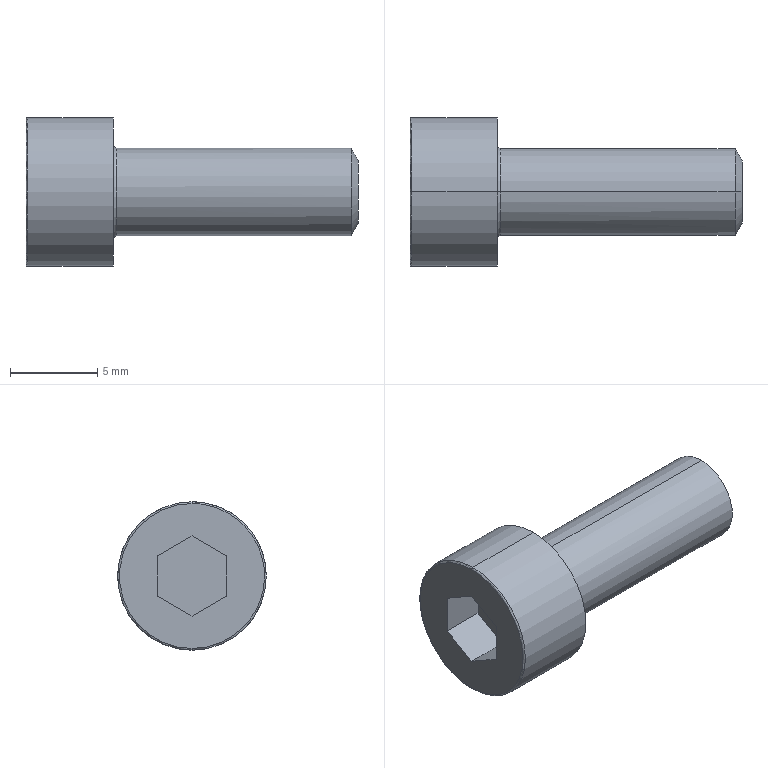Part | STEP file | 103000006185 | 1 solid | 20 faces | box 19 x 8.5 x 8.5 mm | volume 522.658 mm3 | plane 10 | torus 4 | cylinder 4 | cone 2 | commonest cylinder face diameters 5 x2 8.5 x2
STEP:
#1=CARTESIAN_POINT('',(0.,0.,4.15));
#2=VERTEX_POINT('',#1);
#3=CARTESIAN_POINT('',(0.,0.,-4.15));
#4=VERTEX_POINT('',#3);
#5=CARTESIAN_POINT('',(0.,0.,0.));
#6=DIRECTION('',(1.,0.,0.));
#7=AXIS2_PLACEMENT_3D('',#5,#6,$);
#8=CIRCLE('',#7,4.15);
#9=EDGE_CURVE('',#2,#4,#8,.F.);
#10=ORIENTED_EDGE('',*,*,#9,.F.);
#11=CARTESIAN_POINT('',(0.1,0.,4.25));
#12=VERTEX_POINT('',#11);
#13=CARTESIAN_POINT('',(0.1,0.,4.15));
#14=DIRECTION('',(0.,1.,0.));
#15=AXIS2_PLACEMENT_3D('',#13,#14,$);
#16=CIRCLE('',#15,0.1);
#17=EDGE_CURVE('',#2,#12,#16,.T.);
#18=ORIENTED_EDGE('',*,*,#17,.T.);
#19=CARTESIAN_POINT('',(0.1,0.,-4.25));
#20=VERTEX_POINT('',#19);
#21=CARTESIAN_POINT('',(0.1,0.,0.));
#22=DIRECTION('',(1.,0.,0.));
#23=AXIS2_PLACEMENT_3D('',#21,#22,$);
#24=CIRCLE('',#23,4.25);
#25=EDGE_CURVE('',#20,#12,#24,.T.);
#26=ORIENTED_EDGE('',*,*,#25,.F.);
#27=CARTESIAN_POINT('',(0.1,0.,-4.15));
#28=DIRECTION('',(0.,-1.,0.));
#29=AXIS2_PLACEMENT_3D('',#27,#28,$);
#30=CIRCLE('',#29,0.1);
#31=EDGE_CURVE('',#4,#20,#30,.T.);
#32=ORIENTED_EDGE('',*,*,#31,.F.);
#33=EDGE_LOOP('',(#10,#18,#26,#32));
#34=FACE_OUTER_BOUND('',#33,.T.);
#35=CARTESIAN_POINT('',(0.1,0.,0.));
#36=DIRECTION('',(1.,0.,0.));
#37=DIRECTION('',(0.,0.,-1.));
#38=AXIS2_PLACEMENT_3D('',#35,#36,#37);
#39=TOROIDAL_SURFACE('',#38,4.15,0.1);
#40=ADVANCED_FACE('',(#34),#39,.T.);
#41=CARTESIAN_POINT('',(0.,0.,-4.15));
#42=CARTESIAN_POINT('',(0.,-0.3992,-4.15));
#43=CARTESIAN_POINT('',(0.,-0.7984,-4.102));
#44=CARTESIAN_POINT('',(0.,-1.19,-4.006));
#45=CARTESIAN_POINT('',(0.,-1.942,-3.722));
#46=CARTESIAN_POINT('',(0.,-2.606,-3.267));
#47=CARTESIAN_POINT('',(0.,-2.908,-3.001));
#48=CARTESIAN_POINT('',(0.,-3.444,-2.401));
#49=CARTESIAN_POINT('',(0.,-3.821,-1.691));
#50=CARTESIAN_POINT('',(0.,-3.967,-1.315));
#51=CARTESIAN_POINT('',(0.,-4.164,-0.5355));
#52=CARTESIAN_POINT('',(0.,-4.17,0.2686));
#53=CARTESIAN_POINT('',(0.,-4.125,0.6692));
#54=CARTESIAN_POINT('',(0.,-3.939,1.452));
#55=CARTESIAN_POINT('',(0.,-3.573,2.167));
#56=CARTESIAN_POINT('',(0.,-3.347,2.502));
#57=CARTESIAN_POINT('',(0.,-2.821,3.109));
#58=CARTESIAN_POINT('',(0.,-2.165,3.575));
#59=CARTESIAN_POINT('',(0.,-1.81,3.766));
#60=CARTESIAN_POINT('',(0.,-1.237,3.992));
#61=CARTESIAN_POINT('',(0.,-0.6358,4.109));
#62=CARTESIAN_POINT('',(0.,-0.4247,4.136));
#63=CARTESIAN_POINT('',(0.,-0.2123,4.15));
#64=CARTESIAN_POINT('',(0.,0.,4.15));
#65=B_SPLINE_CURVE_WITH_KNOTS('',5,(#41,#42,#43,#44,#45,#46,#47,#48,#49,#50,#51,#52,#53,#54,#55,#56,#57,#58,#59,#60,#61,#62,#63,#64),.UNSPECIFIED.,.F.,.U.,(6,3,3,3,3,3,3,6),(0.,2.823,5.645,8.468,11.291,14.114,16.936,18.438),.UNSPECIFIED.);
#66=EDGE_CURVE('',#4,#2,#65,.T.);
#67=ORIENTED_EDGE('',*,*,#66,.T.);
#68=ORIENTED_EDGE('',*,*,#9,.T.);
#69=EDGE_LOOP('',(#67,#68));
#70=FACE_OUTER_BOUND('',#69,.T.);
#71=CARTESIAN_POINT('',(0.,0.,2.29));
#72=VERTEX_POINT('',#71);
#73=CARTESIAN_POINT('',(0.,1.983,1.145));
#74=VERTEX_POINT('',#73);
#75=CARTESIAN_POINT('',(0.,0.9916,1.717));
#76=DIRECTION('',(0.,0.866,-0.5));
#77=VECTOR('',#76,1.);
#78=LINE('',#75,#77);
#79=EDGE_CURVE('',#72,#74,#78,.T.);
#80=ORIENTED_EDGE('',*,*,#79,.F.);
#81=CARTESIAN_POINT('',(0.,-1.983,1.145));
#82=VERTEX_POINT('',#81);
#83=CARTESIAN_POINT('',(0.,-0.9916,1.717));
#84=DIRECTION('',(0.,0.866,0.5));
#85=VECTOR('',#84,1.);
#86=LINE('',#83,#85);
#87=EDGE_CURVE('',#82,#72,#86,.T.);
#88=ORIENTED_EDGE('',*,*,#87,.F.);
#89=CARTESIAN_POINT('',(0.,-1.983,-1.145));
#90=VERTEX_POINT('',#89);
#91=CARTESIAN_POINT('',(0.,-1.983,0.));
#92=DIRECTION('',(0.,0.,1.));
#93=VECTOR('',#92,1.);
#94=LINE('',#91,#93);
#95=EDGE_CURVE('',#90,#82,#94,.T.);
#96=ORIENTED_EDGE('',*,*,#95,.F.);
#97=CARTESIAN_POINT('',(0.,0.,-2.29));
#98=VERTEX_POINT('',#97);
#99=CARTESIAN_POINT('',(0.,-0.9916,-1.717));
#100=DIRECTION('',(0.,-0.866,0.5));
#101=VECTOR('',#100,1.);
#102=LINE('',#99,#101);
#103=EDGE_CURVE('',#98,#90,#102,.T.);
#104=ORIENTED_EDGE('',*,*,#103,.F.);
#105=CARTESIAN_POINT('',(0.,1.983,-1.145));
#106=VERTEX_POINT('',#105);
#107=CARTESIAN_POINT('',(0.,0.9916,-1.717));
#108=DIRECTION('',(0.,-0.866,-0.5));
#109=VECTOR('',#108,1.);
#110=LINE('',#107,#109);
#111=EDGE_CURVE('',#106,#98,#110,.T.);
#112=ORIENTED_EDGE('',*,*,#111,.F.);
#113=CARTESIAN_POINT('',(0.,1.983,0.));
#114=DIRECTION('',(0.,0.,-1.));
#115=VECTOR('',#114,1.);
#116=LINE('',#113,#115);
#117=EDGE_CURVE('',#74,#106,#116,.T.);
#118=ORIENTED_EDGE('',*,*,#117,.F.);
#119=EDGE_LOOP('',(#80,#88,#96,#104,#112,#118));
#120=FACE_BOUND('',#119,.T.);
#121=CARTESIAN_POINT('',(0.,0.,0.));
#122=DIRECTION('',(1.,0.,0.));
#123=DIRECTION('',(0.,0.,-1.));
#124=AXIS2_PLACEMENT_3D('',#121,#122,#123);
#125=PLANE('',#124);
#126=ADVANCED_FACE('',(#70,#120),#125,.F.);
#127=ORIENTED_EDGE('',*,*,#17,.F.);
#128=ORIENTED_EDGE('',*,*,#66,.F.);
#129=ORIENTED_EDGE('',*,*,#31,.T.);
#130=CARTESIAN_POINT('',(0.1,0.,0.));
#131=DIRECTION('',(1.,0.,0.));
#132=AXIS2_PLACEMENT_3D('',#130,#131,$);
#133=CIRCLE('',#132,4.25);
#134=EDGE_CURVE('',#12,#20,#133,.T.);
#135=ORIENTED_EDGE('',*,*,#134,.F.);
#136=EDGE_LOOP('',(#127,#128,#129,#135));
#137=FACE_OUTER_BOUND('',#136,.T.);
#138=CARTESIAN_POINT('',(0.1,0.,0.));
#139=DIRECTION('',(1.,0.,0.));
#140=DIRECTION('',(0.,0.,1.));
#141=AXIS2_PLACEMENT_3D('',#138,#139,#140);
#142=TOROIDAL_SURFACE('',#141,4.15,0.1);
#143=ADVANCED_FACE('',(#137),#142,.T.);
#144=CARTESIAN_POINT('',(5.,0.,4.25));
#145=VERTEX_POINT('',#144);
#146=CARTESIAN_POINT('',(5.,0.,-4.25));
#147=VERTEX_POINT('',#146);
#148=CARTESIAN_POINT('',(5.,0.,0.));
#149=DIRECTION('',(-1.,0.,0.));
#150=AXIS2_PLACEMENT_3D('',#148,#149,$);
#151=CIRCLE('',#150,4.25);
#152=EDGE_CURVE('',#145,#147,#151,.T.);
#153=ORIENTED_EDGE('',*,*,#152,.T.);
#154=CARTESIAN_POINT('',(0.,0.,-4.25));
#155=DIRECTION('',(-1.,0.,0.));
#156=VECTOR('',#155,1.);
#157=LINE('',#154,#156);
#158=EDGE_CURVE('',#147,#20,#157,.T.);
#159=ORIENTED_EDGE('',*,*,#158,.T.);
#160=ORIENTED_EDGE('',*,*,#25,.T.);
#161=CARTESIAN_POINT('',(0.,0.,4.25));
#162=DIRECTION('',(-1.,0.,0.));
#163=VECTOR('',#162,1.);
#164=LINE('',#161,#163);
#165=EDGE_CURVE('',#145,#12,#164,.T.);
#166=ORIENTED_EDGE('',*,*,#165,.F.);
#167=EDGE_LOOP('',(#153,#159,#160,#166));
#168=FACE_OUTER_BOUND('',#167,.T.);
#169=CARTESIAN_POINT('',(0.,0.,0.));
#170=DIRECTION('',(-1.,0.,0.));
#171=DIRECTION('',(0.,0.,1.));
#172=AXIS2_PLACEMENT_3D('',#169,#170,#171);
#173=CYLINDRICAL_SURFACE('',#172,4.25);
#174=ADVANCED_FACE('',(#168),#173,.T.);
#175=ORIENTED_EDGE('',*,*,#79,.T.);
#176=CARTESIAN_POINT('',(2.5,1.983,1.145));
#177=VERTEX_POINT('',#176);
#178=CARTESIAN_POINT('',(1.25,1.983,1.145));
#179=DIRECTION('',(-1.,0.,0.));
#180=VECTOR('',#179,1.);
#181=LINE('',#178,#180);
#182=EDGE_CURVE('',#177,#74,#181,.T.);
#183=ORIENTED_EDGE('',*,*,#182,.F.);
#184=CARTESIAN_POINT('',(2.5,-0.000000001,2.29));
#185=VERTEX_POINT('',#184);
#186=CARTESIAN_POINT('',(2.5,0.9916,1.718));
#187=DIRECTION('',(0.,0.866,-0.5));
#188=VECTOR('',#187,1.);
#189=LINE('',#186,#188);
#190=EDGE_CURVE('',#185,#177,#189,.T.);
#191=ORIENTED_EDGE('',*,*,#190,.F.);
#192=CARTESIAN_POINT('',(1.25,0.,2.29));
#193=DIRECTION('',(-1.,0.,0.));
#194=VECTOR('',#193,1.);
#195=LINE('',#192,#194);
#196=EDGE_CURVE('',#185,#72,#195,.T.);
#197=ORIENTED_EDGE('',*,*,#196,.T.);
#198=EDGE_LOOP('',(#175,#183,#191,#197));
#199=FACE_OUTER_BOUND('',#198,.T.);
#200=CARTESIAN_POINT('',(2.5,0.,2.29));
#201=DIRECTION('',(0.,0.5,0.866));
#202=DIRECTION('',(0.,-0.866,0.5));
#203=AXIS2_PLACEMENT_3D('',#200,#201,#202);
#204=PLANE('',#203);
#205=ADVANCED_FACE('',(#199),#204,.F.);
#206=ORIENTED_EDGE('',*,*,#87,.T.);
#207=ORIENTED_EDGE('',*,*,#196,.F.);
#208=CARTESIAN_POINT('',(2.5,-1.983,1.145));
#209=VERTEX_POINT('',#208);
#210=CARTESIAN_POINT('',(2.5,-0.9916,1.717));
#211=DIRECTION('',(0.,0.866,0.5));
#212=VECTOR('',#211,1.);
#213=LINE('',#210,#212);
#214=EDGE_CURVE('',#209,#185,#213,.T.);
#215=ORIENTED_EDGE('',*,*,#214,.F.);
#216=CARTESIAN_POINT('',(1.25,-1.983,1.145));
#217=DIRECTION('',(-1.,0.,0.));
#218=VECTOR('',#217,1.);
#219=LINE('',#216,#218);
#220=EDGE_CURVE('',#209,#82,#219,.T.);
#221=ORIENTED_EDGE('',*,*,#220,.T.);
#222=EDGE_LOOP('',(#206,#207,#215,#221));
#223=FACE_OUTER_BOUND('',#222,.T.);
#224=CARTESIAN_POINT('',(2.5,-1.983,1.145));
#225=DIRECTION('',(0.,-0.5,0.866));
#226=DIRECTION('',(0.,-0.866,-0.5));
#227=AXIS2_PLACEMENT_3D('',#224,#225,#226);
#228=PLANE('',#227);
#229=ADVANCED_FACE('',(#223),#228,.F.);
#230=ORIENTED_EDGE('',*,*,#95,.T.);
#231=ORIENTED_EDGE('',*,*,#220,.F.);
#232=CARTESIAN_POINT('',(2.5,-1.983,-1.145));
#233=VERTEX_POINT('',#232);
#234=CARTESIAN_POINT('',(2.5,-1.983,0.));
#235=DIRECTION('',(0.,0.,1.));
#236=VECTOR('',#235,1.);
#237=LINE('',#234,#236);
#238=EDGE_CURVE('',#233,#209,#237,.T.);
#239=ORIENTED_EDGE('',*,*,#238,.F.);
#240=CARTESIAN_POINT('',(1.25,-1.983,-1.145));
#241=DIRECTION('',(-1.,0.,0.));
#242=VECTOR('',#241,1.);
#243=LINE('',#240,#242);
#244=EDGE_CURVE('',#233,#90,#243,.T.);
#245=ORIENTED_EDGE('',*,*,#244,.T.);
#246=EDGE_LOOP('',(#230,#231,#239,#245));
#247=FACE_OUTER_BOUND('',#246,.T.);
#248=CARTESIAN_POINT('',(2.5,-1.983,-1.145));
#249=DIRECTION('',(0.,-1.,0.));
#250=DIRECTION('',(0.,0.,-1.));
#251=AXIS2_PLACEMENT_3D('',#248,#249,#250);
#252=PLANE('',#251);
#253=ADVANCED_FACE('',(#247),#252,.F.);
#254=ORIENTED_EDGE('',*,*,#103,.T.);
#255=ORIENTED_EDGE('',*,*,#244,.F.);
#256=CARTESIAN_POINT('',(2.5,0.,-2.29));
#257=VERTEX_POINT('',#256);
#258=CARTESIAN_POINT('',(2.5,-0.9916,-1.718));
#259=DIRECTION('',(0.,-0.866,0.5));
#260=VECTOR('',#259,1.);
#261=LINE('',#258,#260);
#262=EDGE_CURVE('',#257,#233,#261,.T.);
#263=ORIENTED_EDGE('',*,*,#262,.F.);
#264=CARTESIAN_POINT('',(1.25,0.,-2.29));
#265=DIRECTION('',(-1.,0.,0.));
#266=VECTOR('',#265,1.);
#267=LINE('',#264,#266);
#268=EDGE_CURVE('',#257,#98,#267,.T.);
#269=ORIENTED_EDGE('',*,*,#268,.T.);
#270=EDGE_LOOP('',(#254,#255,#263,#269));
#271=FACE_OUTER_BOUND('',#270,.T.);
#272=CARTESIAN_POINT('',(2.5,0.,-2.29));
#273=DIRECTION('',(0.,-0.5,-0.866));
#274=DIRECTION('',(0.,0.866,-0.5));
#275=AXIS2_PLACEMENT_3D('',#272,#273,#274);
#276=PLANE('',#275);
#277=ADVANCED_FACE('',(#271),#276,.F.);
#278=ORIENTED_EDGE('',*,*,#111,.T.);
#279=ORIENTED_EDGE('',*,*,#268,.F.);
#280=CARTESIAN_POINT('',(2.5,1.983,-1.145));
#281=VERTEX_POINT('',#280);
#282=CARTESIAN_POINT('',(2.5,0.9916,-1.717));
#283=DIRECTION('',(0.,-0.866,-0.5));
#284=VECTOR('',#283,1.);
#285=LINE('',#282,#284);
#286=EDGE_CURVE('',#281,#257,#285,.T.);
#287=ORIENTED_EDGE('',*,*,#286,.F.);
#288=CARTESIAN_POINT('',(1.25,1.983,-1.145));
#289=DIRECTION('',(-1.,0.,0.));
#290=VECTOR('',#289,1.);
#291=LINE('',#288,#290);
#292=EDGE_CURVE('',#281,#106,#291,.T.);
#293=ORIENTED_EDGE('',*,*,#292,.T.);
#294=EDGE_LOOP('',(#278,#279,#287,#293));
#295=FACE_OUTER_BOUND('',#294,.T.);
#296=CARTESIAN_POINT('',(2.5,1.983,-1.145));
#297=DIRECTION('',(0.,0.5,-0.866));
#298=DIRECTION('',(0.,0.866,0.5));
#299=AXIS2_PLACEMENT_3D('',#296,#297,#298);
#300=PLANE('',#299);
#301=ADVANCED_FACE('',(#295),#300,.F.);
#302=ORIENTED_EDGE('',*,*,#117,.T.);
#303=ORIENTED_EDGE('',*,*,#292,.F.);
#304=CARTESIAN_POINT('',(2.5,1.983,0.));
#305=DIRECTION('',(0.,0.,-1.));
#306=VECTOR('',#305,1.);
#307=LINE('',#304,#306);
#308=EDGE_CURVE('',#177,#281,#307,.T.);
#309=ORIENTED_EDGE('',*,*,#308,.F.);
#310=ORIENTED_EDGE('',*,*,#182,.T.);
#311=EDGE_LOOP('',(#302,#303,#309,#310));
#312=FACE_OUTER_BOUND('',#311,.T.);
#313=CARTESIAN_POINT('',(2.5,1.983,1.145));
#314=DIRECTION('',(0.,1.,0.));
#315=DIRECTION('',(0.,0.,1.));
#316=AXIS2_PLACEMENT_3D('',#313,#314,#315);
#317=PLANE('',#316);
#318=ADVANCED_FACE('',(#312),#317,.F.);
#319=ORIENTED_EDGE('',*,*,#158,.F.);
#320=CARTESIAN_POINT('',(5.,0.,0.));
#321=DIRECTION('',(-1.,0.,0.));
#322=AXIS2_PLACEMENT_3D('',#320,#321,$);
#323=CIRCLE('',#322,4.25);
#324=EDGE_CURVE('',#147,#145,#323,.T.);
#325=ORIENTED_EDGE('',*,*,#324,.T.);
#326=ORIENTED_EDGE('',*,*,#165,.T.);
#327=ORIENTED_EDGE('',*,*,#134,.T.);
#328=EDGE_LOOP('',(#319,#325,#326,#327));
#329=FACE_OUTER_BOUND('',#328,.T.);
#330=CARTESIAN_POINT('',(0.,0.,0.));
#331=DIRECTION('',(-1.,0.,0.));
#332=DIRECTION('',(0.,0.,-1.));
#333=AXIS2_PLACEMENT_3D('',#330,#331,#332);
#334=CYLINDRICAL_SURFACE('',#333,4.25);
#335=ADVANCED_FACE('',(#329),#334,.T.);
#336=ORIENTED_EDGE('',*,*,#152,.F.);
#337=ORIENTED_EDGE('',*,*,#324,.F.);
#338=EDGE_LOOP('',(#336,#337));
#339=FACE_OUTER_BOUND('',#338,.T.);
#340=CARTESIAN_POINT('',(5.,0.,2.7));
#341=VERTEX_POINT('',#340);
#342=CARTESIAN_POINT('',(5.,0.,-2.7));
#343=VERTEX_POINT('',#342);
#344=CARTESIAN_POINT('',(5.,0.,0.));
#345=DIRECTION('',(-1.,0.,0.));
#346=AXIS2_PLACEMENT_3D('',#344,#345,$);
#347=CIRCLE('',#346,2.7);
#348=EDGE_CURVE('',#341,#343,#347,.T.);
#349=ORIENTED_EDGE('',*,*,#348,.T.);
#350=CARTESIAN_POINT('',(5.,0.,0.));
#351=DIRECTION('',(-1.,0.,0.));
#352=AXIS2_PLACEMENT_3D('',#350,#351,$);
#353=CIRCLE('',#352,2.7);
#354=EDGE_CURVE('',#343,#341,#353,.T.);
#355=ORIENTED_EDGE('',*,*,#354,.T.);
#356=EDGE_LOOP('',(#349,#355));
#357=FACE_BOUND('',#356,.T.);
#358=CARTESIAN_POINT('',(5.,4.25,0.));
#359=DIRECTION('',(-1.,0.,0.));
#360=DIRECTION('',(0.,0.,1.));
#361=AXIS2_PLACEMENT_3D('',#358,#359,#360);
#362=PLANE('',#361);
#363=ADVANCED_FACE('',(#339,#357),#362,.F.);
#364=ORIENTED_EDGE('',*,*,#214,.T.);
#365=ORIENTED_EDGE('',*,*,#190,.T.);
#366=ORIENTED_EDGE('',*,*,#308,.T.);
#367=ORIENTED_EDGE('',*,*,#286,.T.);
#368=ORIENTED_EDGE('',*,*,#262,.T.);
#369=ORIENTED_EDGE('',*,*,#238,.T.);
#370=EDGE_LOOP('',(#364,#365,#366,#367,#368,#369));
#371=FACE_OUTER_BOUND('',#370,.T.);
#372=CARTESIAN_POINT('',(2.5,-1.983,1.145));
#373=DIRECTION('',(1.,0.,0.));
#374=DIRECTION('',(0.,0.,-1.));
#375=AXIS2_PLACEMENT_3D('',#372,#373,#374);
#376=PLANE('',#375);
#377=ADVANCED_FACE('',(#371),#376,.F.);
#378=CARTESIAN_POINT('',(5.2,0.,-2.5));
#379=VERTEX_POINT('',#378);
#380=CARTESIAN_POINT('',(5.2,0.,-2.7));
#381=DIRECTION('',(0.,1.,0.));
#382=AXIS2_PLACEMENT_3D('',#380,#381,$);
#383=CIRCLE('',#382,0.2);
#384=EDGE_CURVE('',#343,#379,#383,.T.);
#385=ORIENTED_EDGE('',*,*,#384,.F.);
#386=ORIENTED_EDGE('',*,*,#348,.F.);
#387=CARTESIAN_POINT('',(5.2,0.,2.5));
#388=VERTEX_POINT('',#387);
#389=CARTESIAN_POINT('',(5.2,0.,2.7));
#390=DIRECTION('',(0.,-1.,0.));
#391=AXIS2_PLACEMENT_3D('',#389,#390,$);
#392=CIRCLE('',#391,0.2);
#393=EDGE_CURVE('',#341,#388,#392,.T.);
#394=ORIENTED_EDGE('',*,*,#393,.T.);
#395=CARTESIAN_POINT('',(5.2,0.,0.));
#396=DIRECTION('',(-1.,0.,0.));
#397=AXIS2_PLACEMENT_3D('',#395,#396,$);
#398=CIRCLE('',#397,2.5);
#399=EDGE_CURVE('',#388,#379,#398,.T.);
#400=ORIENTED_EDGE('',*,*,#399,.T.);
#401=EDGE_LOOP('',(#385,#386,#394,#400));
#402=FACE_OUTER_BOUND('',#401,.T.);
#403=CARTESIAN_POINT('',(5.2,0.,0.));
#404=DIRECTION('',(-1.,0.,0.));
#405=DIRECTION('',(0.,0.,1.));
#406=AXIS2_PLACEMENT_3D('',#403,#404,#405);
#407=TOROIDAL_SURFACE('',#406,2.7,0.2);
#408=ADVANCED_FACE('',(#402),#407,.F.);
#409=ORIENTED_EDGE('',*,*,#354,.F.);
#410=ORIENTED_EDGE('',*,*,#384,.T.);
#411=CARTESIAN_POINT('',(5.2,0.,0.));
#412=DIRECTION('',(-1.,0.,0.));
#413=AXIS2_PLACEMENT_3D('',#411,#412,$);
#414=CIRCLE('',#413,2.5);
#415=EDGE_CURVE('',#379,#388,#414,.T.);
#416=ORIENTED_EDGE('',*,*,#415,.T.);
#417=ORIENTED_EDGE('',*,*,#393,.F.);
#418=EDGE_LOOP('',(#409,#410,#416,#417));
#419=FACE_OUTER_BOUND('',#418,.T.);
#420=CARTESIAN_POINT('',(5.2,0.,0.));
#421=DIRECTION('',(-1.,0.,0.));
#422=DIRECTION('',(0.,0.,-1.));
#423=AXIS2_PLACEMENT_3D('',#420,#421,#422);
#424=TOROIDAL_SURFACE('',#423,2.7,0.2);
#425=ADVANCED_FACE('',(#419),#424,.F.);
#426=CARTESIAN_POINT('',(18.6,0.,2.5));
#427=VERTEX_POINT('',#426);
#428=CARTESIAN_POINT('',(18.6,0.,-2.5));
#429=VERTEX_POINT('',#428);
#430=CARTESIAN_POINT('',(18.6,0.,0.));
#431=DIRECTION('',(-1.,0.,0.));
#432=AXIS2_PLACEMENT_3D('',#430,#431,$);
#433=CIRCLE('',#432,2.5);
#434=EDGE_CURVE('',#427,#429,#433,.T.);
#435=ORIENTED_EDGE('',*,*,#434,.T.);
#436=CARTESIAN_POINT('',(0.,0.,-2.5));
#437=DIRECTION('',(-1.,0.,0.));
#438=VECTOR('',#437,1.);
#439=LINE('',#436,#438);
#440=EDGE_CURVE('',#429,#379,#439,.T.);
#441=ORIENTED_EDGE('',*,*,#440,.T.);
#442=ORIENTED_EDGE('',*,*,#399,.F.);
#443=CARTESIAN_POINT('',(0.,0.,2.5));
#444=DIRECTION('',(-1.,0.,0.));
#445=VECTOR('',#444,1.);
#446=LINE('',#443,#445);
#447=EDGE_CURVE('',#427,#388,#446,.T.);
#448=ORIENTED_EDGE('',*,*,#447,.F.);
#449=EDGE_LOOP('',(#435,#441,#442,#448));
#450=FACE_OUTER_BOUND('',#449,.T.);
#451=CARTESIAN_POINT('',(0.,0.,0.));
#452=DIRECTION('',(-1.,0.,0.));
#453=DIRECTION('',(0.,0.,1.));
#454=AXIS2_PLACEMENT_3D('',#451,#452,#453);
#455=CYLINDRICAL_SURFACE('',#454,2.5);
#456=ADVANCED_FACE('',(#450),#455,.T.);
#457=ORIENTED_EDGE('',*,*,#440,.F.);
#458=CARTESIAN_POINT('',(18.6,0.,-2.5));
#459=CARTESIAN_POINT('',(18.6,-0.7854,-2.5));
#460=CARTESIAN_POINT('',(18.6,-1.571,-2.192));
#461=CARTESIAN_POINT('',(18.6,-2.192,-1.571));
#462=CARTESIAN_POINT('',(18.6,-2.808,0.));
#463=CARTESIAN_POINT('',(18.6,-2.192,1.571));
#464=CARTESIAN_POINT('',(18.6,-1.571,2.192));
#465=CARTESIAN_POINT('',(18.6,-0.7854,2.5));
#466=CARTESIAN_POINT('',(18.6,0.,2.5));
#467=B_SPLINE_CURVE_WITH_KNOTS('',5,(#458,#459,#460,#461,#462,#463,#464,#465,#466),.UNSPECIFIED.,.F.,.U.,(6,3,6),(-3.927,0.,3.927),.UNSPECIFIED.);
#468=EDGE_CURVE('',#429,#427,#467,.T.);
#469=ORIENTED_EDGE('',*,*,#468,.T.);
#470=ORIENTED_EDGE('',*,*,#447,.T.);
#471=ORIENTED_EDGE('',*,*,#415,.F.);
#472=EDGE_LOOP('',(#457,#469,#470,#471));
#473=FACE_OUTER_BOUND('',#472,.T.);
#474=CARTESIAN_POINT('',(0.,0.,0.));
#475=DIRECTION('',(-1.,0.,0.));
#476=DIRECTION('',(0.,0.,-1.));
#477=AXIS2_PLACEMENT_3D('',#474,#475,#476);
#478=CYLINDRICAL_SURFACE('',#477,2.5);
#479=ADVANCED_FACE('',(#473),#478,.T.);
#480=CARTESIAN_POINT('',(19.,0.,1.807));
#481=VERTEX_POINT('',#480);
#482=CARTESIAN_POINT('',(19.,0.,-1.807));
#483=VERTEX_POINT('',#482);
#484=CARTESIAN_POINT('',(19.,0.,0.));
#485=DIRECTION('',(-1.,0.,0.));
#486=AXIS2_PLACEMENT_3D('',#484,#485,$);
#487=CIRCLE('',#486,1.807);
#488=EDGE_CURVE('',#481,#483,#487,.T.);
#489=ORIENTED_EDGE('',*,*,#488,.T.);
#490=CARTESIAN_POINT('',(-249980.678,0.,-433013.952));
#491=DIRECTION('',(-0.5,0.,-0.866));
#492=VECTOR('',#491,1.);
#493=LINE('',#490,#492);
#494=EDGE_CURVE('',#483,#429,#493,.T.);
#495=ORIENTED_EDGE('',*,*,#494,.T.);
#496=ORIENTED_EDGE('',*,*,#434,.F.);
#497=CARTESIAN_POINT('',(-249980.678,0.,433013.952));
#498=DIRECTION('',(-0.5,0.,0.866));
#499=VECTOR('',#498,1.);
#500=LINE('',#497,#499);
#501=EDGE_CURVE('',#481,#427,#500,.T.);
#502=ORIENTED_EDGE('',*,*,#501,.F.);
#503=EDGE_LOOP('',(#489,#495,#496,#502));
#504=FACE_OUTER_BOUND('',#503,.T.);
#505=CARTESIAN_POINT('',(18.6,0.,0.));
#506=DIRECTION('',(-1.,0.,0.));
#507=DIRECTION('',(0.,0.,1.));
#508=AXIS2_PLACEMENT_3D('',#505,#506,#507);
#509=CONICAL_SURFACE('',#508,2.5,1.047);
#510=ADVANCED_FACE('',(#504),#509,.T.);
#511=ORIENTED_EDGE('',*,*,#494,.F.);
#512=CARTESIAN_POINT('',(19.,0.,0.));
#513=DIRECTION('',(-1.,0.,0.));
#514=AXIS2_PLACEMENT_3D('',#512,#513,$);
#515=CIRCLE('',#514,1.807);
#516=EDGE_CURVE('',#483,#481,#515,.T.);
#517=ORIENTED_EDGE('',*,*,#516,.T.);
#518=ORIENTED_EDGE('',*,*,#501,.T.);
#519=ORIENTED_EDGE('',*,*,#468,.F.);
#520=EDGE_LOOP('',(#511,#517,#518,#519));
#521=FACE_OUTER_BOUND('',#520,.T.);
#522=CARTESIAN_POINT('',(18.6,0.,0.));
#523=DIRECTION('',(-1.,0.,0.));
#524=DIRECTION('',(0.,0.,-1.));
#525=AXIS2_PLACEMENT_3D('',#522,#523,#524);
#526=CONICAL_SURFACE('',#525,2.5,1.047);
#527=ADVANCED_FACE('',(#521),#526,.T.);
#528=ORIENTED_EDGE('',*,*,#488,.F.);
#529=ORIENTED_EDGE('',*,*,#516,.F.);
#530=EDGE_LOOP('',(#528,#529));
#531=FACE_OUTER_BOUND('',#530,.T.);
#532=CARTESIAN_POINT('',(19.,2.5,0.));
#533=DIRECTION('',(-1.,0.,0.));
#534=DIRECTION('',(0.,0.,1.));
#535=AXIS2_PLACEMENT_3D('',#532,#533,#534);
#536=PLANE('',#535);
#537=ADVANCED_FACE('',(#531),#536,.F.);
#538=CLOSED_SHELL('',(#40,#126,#143,#174,#205,#229,#253,#277,#301,#318,#335,#363,#377,#408,#425,#456,#479,#510,#527,#537));
#539=MANIFOLD_SOLID_BREP('',#538);
#540=(LENGTH_UNIT()NAMED_UNIT(*)SI_UNIT(.MILLI.,.METRE.));
#541=UNCERTAINTY_MEASURE_WITH_UNIT(LENGTH_MEASURE(0.005),#540,'','');
#542=(NAMED_UNIT(*)PLANE_ANGLE_UNIT()SI_UNIT($,.RADIAN.));
#543=(NAMED_UNIT(*)SI_UNIT($,.STERADIAN.)SOLID_ANGLE_UNIT());
#544=(GEOMETRIC_REPRESENTATION_CONTEXT(3)GLOBAL_UNCERTAINTY_ASSIGNED_CONTEXT((#541))GLOBAL_UNIT_ASSIGNED_CONTEXT((#540,#542,#543))REPRESENTATION_CONTEXT('',''));
#545=ADVANCED_BREP_SHAPE_REPRESENTATION('',(#539),#544);